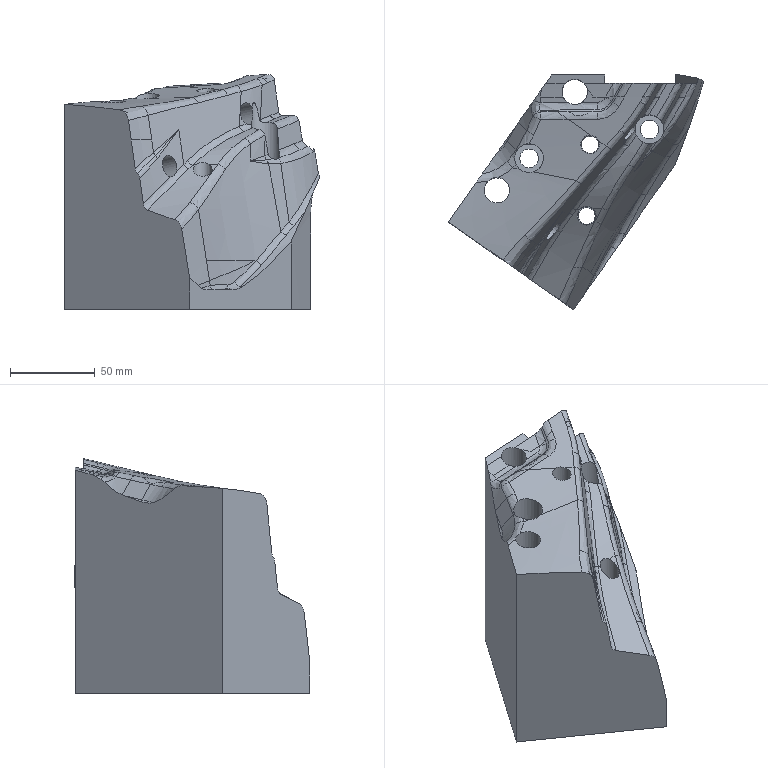Part | NX | features solid 2 | 1 solid | 137 faces | box 150.321 x 138.916 x 138.635 mm | volume 1044307 mm3 | spline 105 | cylinder 16 | plane 16 | commonest cylinder face diameters 10 x4 11 x4 9 x2 13 x2 15 x2 17 x2